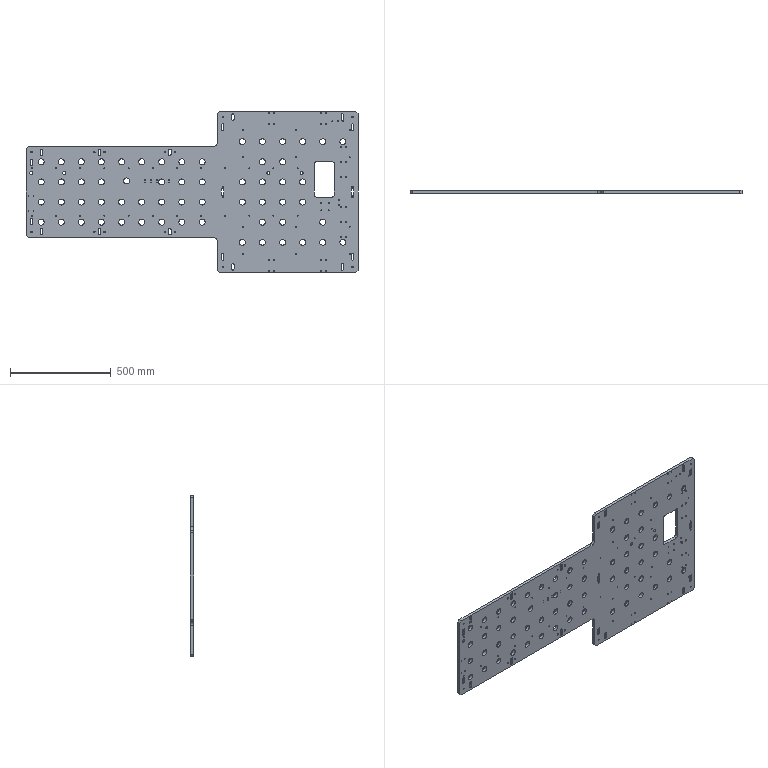Part | NX | 1 solid | 379 faces | box 1650 x 15 x 800 mm | volume 13695332 mm3 | cylinder 257 | plane 122 | commonest cylinder face diameters 30 x60 5 x41 20 x40 12.5 x36 4.2 x24 6.8 x18